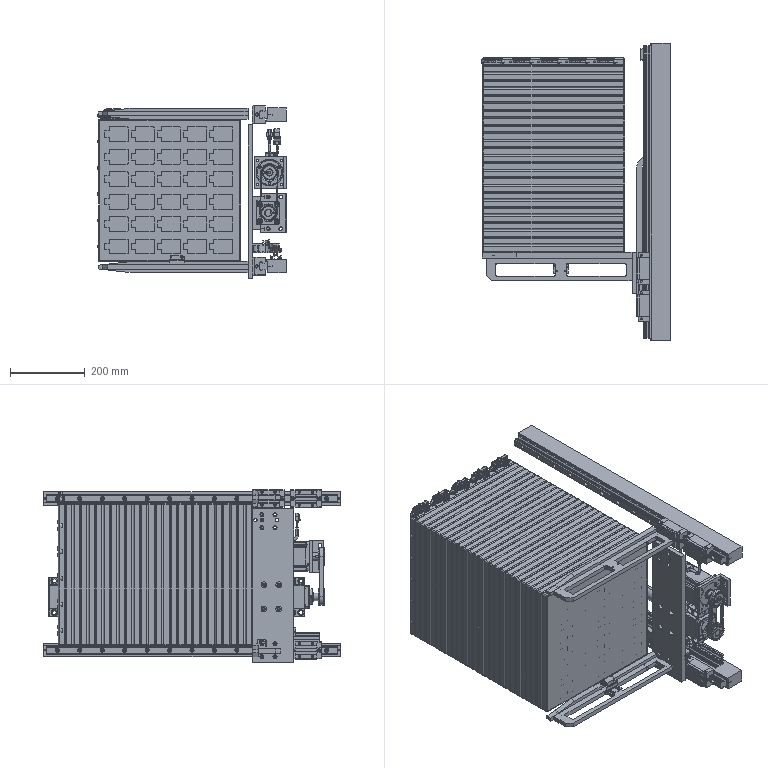Part | SolidWorks | features ReferencePattern 75, LocalLPattern 6, AEMSimFeature 1, CompositeCurve 1 | 144 solids | 68082 faces | volume 53088556 mm3 | cylinder 29610 | spline 15933 | plane 15632 | torus 6278 | cone 421 | sphere 208 | commonest cylinder face diameters 0.6 x15143 6 x8366 2 x889 1 x732 11 x414 6.5 x376